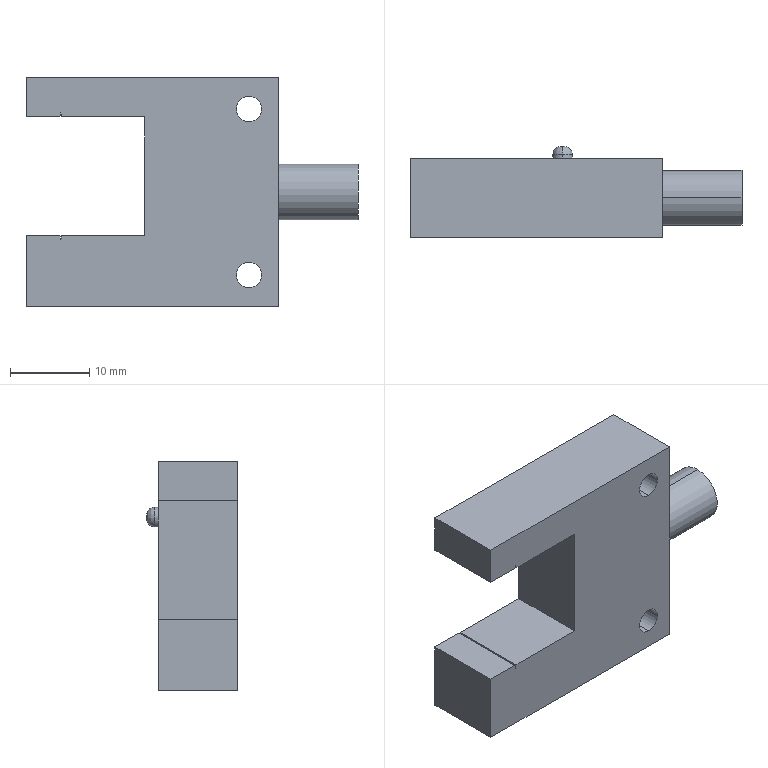Part | STEP file | Photoelectric sensor SU15-N | 1 solid | 42 faces | box 42 x 11.5 x 29 mm | volume 7150 mm3 | plane 32 | cylinder 8 | other 2 | commonest cylinder face diameters 3.2 x4 2.5 x2 7 x2